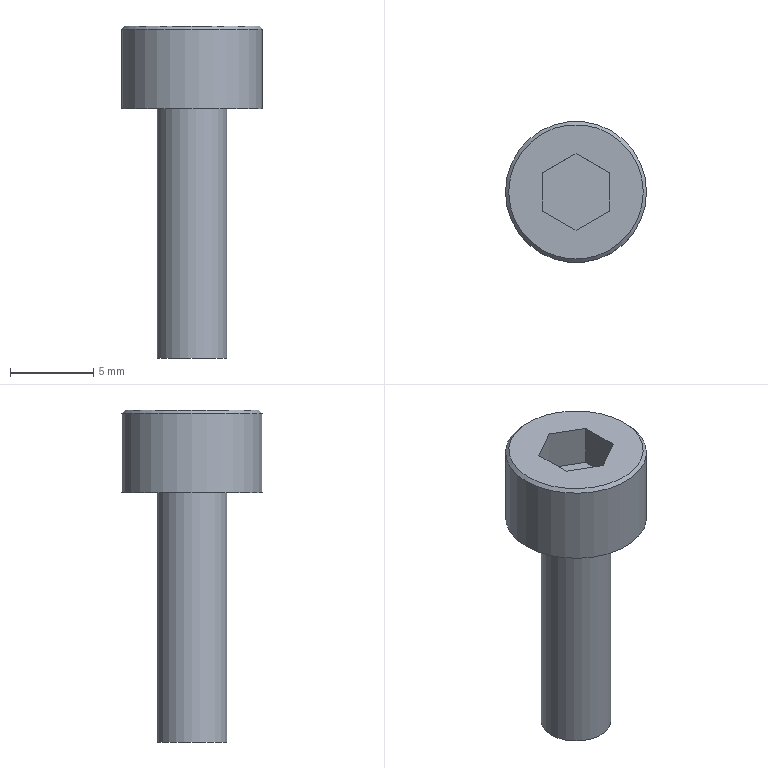Part | STEP file | M3-10_id34_x_t | 1 solid | 13 faces | box 8.5 x 8.5 x 20 mm | volume 456.375 mm3 | plane 10 | cylinder 2 | cone 1 | commonest cylinder face diameters 4.2 x1 8.5 x1
STEP:
#1=CARTESIAN_POINT('',(-234.55,-47.,-11.));
#2=VERTEX_POINT('',#1);
#3=CARTESIAN_POINT('',(-232.45,-47.,-11.));
#4=DIRECTION('',(0.,0.,-1.));
#5=DIRECTION('',(-1.,0.,0.));
#6=AXIS2_PLACEMENT_3D('',#3,#4,#5);
#7=CIRCLE('',#6,2.1);
#8=EDGE_CURVE('',#2,#2,#7,.T.);
#9=ORIENTED_EDGE('',*,*,#8,.F.);
#10=EDGE_LOOP('',(#9));
#11=FACE_BOUND('',#10,.T.);
#12=CARTESIAN_POINT('',(-228.2,-47.,-11.));
#13=VERTEX_POINT('',#12);
#14=CARTESIAN_POINT('',(-232.45,-47.,-11.));
#15=DIRECTION('',(0.,0.,1.));
#16=DIRECTION('',(1.,0.,0.));
#17=AXIS2_PLACEMENT_3D('',#14,#15,#16);
#18=CIRCLE('',#17,4.25);
#19=EDGE_CURVE('',#13,#13,#18,.T.);
#20=ORIENTED_EDGE('',*,*,#19,.F.);
#21=EDGE_LOOP('',(#20));
#22=FACE_BOUND('',#21,.T.);
#23=CARTESIAN_POINT('',(-232.45,-47.,-11.));
#24=DIRECTION('',(0.,0.,-1.));
#25=DIRECTION('',(-1.,0.,0.));
#26=AXIS2_PLACEMENT_3D('',#23,#24,#25);
#27=PLANE('',#26);
#28=ADVANCED_FACE('',(#11,#22),#27,.T.);
#29=CARTESIAN_POINT('',(-230.35,-47.,-26.));
#30=VERTEX_POINT('',#29);
#31=CARTESIAN_POINT('',(-232.45,-47.,-26.));
#32=DIRECTION('',(0.,0.,1.));
#33=DIRECTION('',(1.,0.,0.));
#34=AXIS2_PLACEMENT_3D('',#31,#32,#33);
#35=CIRCLE('',#34,2.1);
#36=EDGE_CURVE('',#30,#30,#35,.T.);
#37=ORIENTED_EDGE('',*,*,#36,.F.);
#38=EDGE_LOOP('',(#37));
#39=FACE_OUTER_BOUND('',#38,.T.);
#40=CARTESIAN_POINT('',(-232.45,-47.,-26.));
#41=DIRECTION('',(0.,0.,-1.));
#42=DIRECTION('',(-1.,0.,0.));
#43=AXIS2_PLACEMENT_3D('',#40,#41,#42);
#44=PLANE('',#43);
#45=ADVANCED_FACE('',(#39),#44,.T.);
#46=ORIENTED_EDGE('',*,*,#36,.T.);
#47=EDGE_LOOP('',(#46));
#48=FACE_BOUND('',#47,.T.);
#49=ORIENTED_EDGE('',*,*,#8,.T.);
#50=EDGE_LOOP('',(#49));
#51=FACE_BOUND('',#50,.T.);
#52=CARTESIAN_POINT('',(-232.45,-47.,-16.));
#53=DIRECTION('',(0.,0.,-1.));
#54=DIRECTION('',(1.,0.,0.));
#55=AXIS2_PLACEMENT_3D('',#52,#53,#54);
#56=CYLINDRICAL_SURFACE('',#55,2.1);
#57=ADVANCED_FACE('',(#48,#51),#56,.T.);
#58=CARTESIAN_POINT('',(-234.45,-45.845,-6.));
#59=VERTEX_POINT('',#58);
#60=CARTESIAN_POINT('',(-234.45,-48.155,-6.));
#61=VERTEX_POINT('',#60);
#62=CARTESIAN_POINT('',(-234.45,-45.845,-6.));
#63=DIRECTION('',(0.,-1.,0.));
#64=VECTOR('',#63,1.);
#65=LINE('',#62,#64);
#66=EDGE_CURVE('',#59,#61,#65,.T.);
#67=ORIENTED_EDGE('',*,*,#66,.F.);
#68=CARTESIAN_POINT('',(-232.45,-44.691,-6.));
#69=VERTEX_POINT('',#68);
#70=CARTESIAN_POINT('',(-232.45,-44.691,-6.));
#71=DIRECTION('',(-0.866,-0.5,0.));
#72=VECTOR('',#71,1.);
#73=LINE('',#70,#72);
#74=EDGE_CURVE('',#69,#59,#73,.T.);
#75=ORIENTED_EDGE('',*,*,#74,.F.);
#76=CARTESIAN_POINT('',(-230.45,-45.845,-6.));
#77=VERTEX_POINT('',#76);
#78=CARTESIAN_POINT('',(-230.45,-45.845,-6.));
#79=DIRECTION('',(-0.866,0.5,0.));
#80=VECTOR('',#79,1.);
#81=LINE('',#78,#80);
#82=EDGE_CURVE('',#77,#69,#81,.T.);
#83=ORIENTED_EDGE('',*,*,#82,.F.);
#84=CARTESIAN_POINT('',(-230.45,-48.155,-6.));
#85=VERTEX_POINT('',#84);
#86=CARTESIAN_POINT('',(-230.45,-48.155,-6.));
#87=DIRECTION('',(0.,1.,0.));
#88=VECTOR('',#87,1.);
#89=LINE('',#86,#88);
#90=EDGE_CURVE('',#85,#77,#89,.T.);
#91=ORIENTED_EDGE('',*,*,#90,.F.);
#92=CARTESIAN_POINT('',(-232.45,-49.309,-6.));
#93=VERTEX_POINT('',#92);
#94=CARTESIAN_POINT('',(-232.45,-49.309,-6.));
#95=DIRECTION('',(0.866,0.5,0.));
#96=VECTOR('',#95,1.);
#97=LINE('',#94,#96);
#98=EDGE_CURVE('',#93,#85,#97,.T.);
#99=ORIENTED_EDGE('',*,*,#98,.F.);
#100=CARTESIAN_POINT('',(-234.45,-48.155,-6.));
#101=DIRECTION('',(0.866,-0.5,0.));
#102=VECTOR('',#101,1.);
#103=LINE('',#100,#102);
#104=EDGE_CURVE('',#61,#93,#103,.T.);
#105=ORIENTED_EDGE('',*,*,#104,.F.);
#106=EDGE_LOOP('',(#67,#75,#83,#91,#99,#105));
#107=FACE_BOUND('',#106,.T.);
#108=CARTESIAN_POINT('',(-228.4,-47.,-6.));
#109=VERTEX_POINT('',#108);
#110=CARTESIAN_POINT('',(-232.45,-47.,-6.));
#111=DIRECTION('',(0.,0.,1.));
#112=DIRECTION('',(1.,0.,0.));
#113=AXIS2_PLACEMENT_3D('',#110,#111,#112);
#114=CIRCLE('',#113,4.05);
#115=EDGE_CURVE('',#109,#109,#114,.T.);
#116=ORIENTED_EDGE('',*,*,#115,.T.);
#117=EDGE_LOOP('',(#116));
#118=FACE_BOUND('',#117,.T.);
#119=CARTESIAN_POINT('',(-232.45,-47.,-6.));
#120=DIRECTION('',(0.,0.,1.));
#121=DIRECTION('',(1.,0.,0.));
#122=AXIS2_PLACEMENT_3D('',#119,#120,#121);
#123=PLANE('',#122);
#124=ADVANCED_FACE('',(#107,#118),#123,.T.);
#125=CARTESIAN_POINT('',(-228.2,-47.,-6.2));
#126=VERTEX_POINT('',#125);
#127=CARTESIAN_POINT('',(-232.45,-47.,-6.2));
#128=DIRECTION('',(0.,0.,-1.));
#129=DIRECTION('',(1.,0.,0.));
#130=AXIS2_PLACEMENT_3D('',#127,#128,#129);
#131=CIRCLE('',#130,4.25);
#132=EDGE_CURVE('',#126,#126,#131,.T.);
#133=ORIENTED_EDGE('',*,*,#132,.T.);
#134=EDGE_LOOP('',(#133));
#135=FACE_BOUND('',#134,.T.);
#136=ORIENTED_EDGE('',*,*,#19,.T.);
#137=EDGE_LOOP('',(#136));
#138=FACE_BOUND('',#137,.T.);
#139=CARTESIAN_POINT('',(-232.45,-47.,-11.));
#140=DIRECTION('',(0.,0.,1.));
#141=DIRECTION('',(1.,0.,0.));
#142=AXIS2_PLACEMENT_3D('',#139,#140,#141);
#143=CYLINDRICAL_SURFACE('',#142,4.25);
#144=ADVANCED_FACE('',(#135,#138),#143,.T.);
#145=ORIENTED_EDGE('',*,*,#115,.F.);
#146=EDGE_LOOP('',(#145));
#147=FACE_BOUND('',#146,.T.);
#148=ORIENTED_EDGE('',*,*,#132,.F.);
#149=EDGE_LOOP('',(#148));
#150=FACE_BOUND('',#149,.T.);
#151=CARTESIAN_POINT('',(-232.45,-47.,-6.2));
#152=DIRECTION('',(0.,0.,-1.));
#153=DIRECTION('',(-1.,0.,0.));
#154=AXIS2_PLACEMENT_3D('',#151,#152,#153);
#155=CONICAL_SURFACE('',#154,4.25,45.);
#156=ADVANCED_FACE('',(#147,#150),#155,.T.);
#157=ORIENTED_EDGE('',*,*,#66,.T.);
#158=CARTESIAN_POINT('',(-234.45,-48.155,-8.5));
#159=VERTEX_POINT('',#158);
#160=CARTESIAN_POINT('',(-234.45,-48.155,-8.5));
#161=DIRECTION('',(0.,0.,-1.));
#162=VECTOR('',#161,1.);
#163=LINE('',#160,#162);
#164=EDGE_CURVE('',#61,#159,#163,.T.);
#165=ORIENTED_EDGE('',*,*,#164,.T.);
#166=CARTESIAN_POINT('',(-234.45,-45.845,-8.5));
#167=VERTEX_POINT('',#166);
#168=CARTESIAN_POINT('',(-234.45,-45.845,-8.5));
#169=DIRECTION('',(0.,1.,0.));
#170=VECTOR('',#169,1.);
#171=LINE('',#168,#170);
#172=EDGE_CURVE('',#159,#167,#171,.T.);
#173=ORIENTED_EDGE('',*,*,#172,.T.);
#174=CARTESIAN_POINT('',(-234.45,-45.845,-8.5));
#175=DIRECTION('',(0.,0.,-1.));
#176=VECTOR('',#175,1.);
#177=LINE('',#174,#176);
#178=EDGE_CURVE('',#59,#167,#177,.T.);
#179=ORIENTED_EDGE('',*,*,#178,.F.);
#180=EDGE_LOOP('',(#157,#165,#173,#179));
#181=FACE_OUTER_BOUND('',#180,.T.);
#182=CARTESIAN_POINT('',(-234.45,-45.845,-8.5));
#183=DIRECTION('',(-1.,0.,0.));
#184=DIRECTION('',(0.,-1.,0.));
#185=AXIS2_PLACEMENT_3D('',#182,#183,#184);
#186=PLANE('',#185);
#187=ADVANCED_FACE('',(#181),#186,.F.);
#188=ORIENTED_EDGE('',*,*,#104,.T.);
#189=CARTESIAN_POINT('',(-232.45,-49.309,-8.5));
#190=VERTEX_POINT('',#189);
#191=CARTESIAN_POINT('',(-232.45,-49.309,-8.5));
#192=DIRECTION('',(0.,0.,-1.));
#193=VECTOR('',#192,1.);
#194=LINE('',#191,#193);
#195=EDGE_CURVE('',#93,#190,#194,.T.);
#196=ORIENTED_EDGE('',*,*,#195,.T.);
#197=CARTESIAN_POINT('',(-234.45,-48.155,-8.5));
#198=DIRECTION('',(-0.866,0.5,0.));
#199=VECTOR('',#198,1.);
#200=LINE('',#197,#199);
#201=EDGE_CURVE('',#190,#159,#200,.T.);
#202=ORIENTED_EDGE('',*,*,#201,.T.);
#203=ORIENTED_EDGE('',*,*,#164,.F.);
#204=EDGE_LOOP('',(#188,#196,#202,#203));
#205=FACE_OUTER_BOUND('',#204,.T.);
#206=CARTESIAN_POINT('',(-234.45,-48.155,-8.5));
#207=DIRECTION('',(-0.5,-0.866,0.));
#208=DIRECTION('',(0.866,-0.5,0.));
#209=AXIS2_PLACEMENT_3D('',#206,#207,#208);
#210=PLANE('',#209);
#211=ADVANCED_FACE('',(#205),#210,.F.);
#212=ORIENTED_EDGE('',*,*,#98,.T.);
#213=CARTESIAN_POINT('',(-230.45,-48.155,-8.5));
#214=VERTEX_POINT('',#213);
#215=CARTESIAN_POINT('',(-230.45,-48.155,-8.5));
#216=DIRECTION('',(0.,0.,-1.));
#217=VECTOR('',#216,1.);
#218=LINE('',#215,#217);
#219=EDGE_CURVE('',#85,#214,#218,.T.);
#220=ORIENTED_EDGE('',*,*,#219,.T.);
#221=CARTESIAN_POINT('',(-232.45,-49.309,-8.5));
#222=DIRECTION('',(-0.866,-0.5,0.));
#223=VECTOR('',#222,1.);
#224=LINE('',#221,#223);
#225=EDGE_CURVE('',#214,#190,#224,.T.);
#226=ORIENTED_EDGE('',*,*,#225,.T.);
#227=ORIENTED_EDGE('',*,*,#195,.F.);
#228=EDGE_LOOP('',(#212,#220,#226,#227));
#229=FACE_OUTER_BOUND('',#228,.T.);
#230=CARTESIAN_POINT('',(-232.45,-49.309,-8.5));
#231=DIRECTION('',(0.5,-0.866,0.));
#232=DIRECTION('',(0.866,0.5,0.));
#233=AXIS2_PLACEMENT_3D('',#230,#231,#232);
#234=PLANE('',#233);
#235=ADVANCED_FACE('',(#229),#234,.F.);
#236=ORIENTED_EDGE('',*,*,#90,.T.);
#237=CARTESIAN_POINT('',(-230.45,-45.845,-8.5));
#238=VERTEX_POINT('',#237);
#239=CARTESIAN_POINT('',(-230.45,-45.845,-8.5));
#240=DIRECTION('',(0.,0.,-1.));
#241=VECTOR('',#240,1.);
#242=LINE('',#239,#241);
#243=EDGE_CURVE('',#77,#238,#242,.T.);
#244=ORIENTED_EDGE('',*,*,#243,.T.);
#245=CARTESIAN_POINT('',(-230.45,-48.155,-8.5));
#246=DIRECTION('',(0.,-1.,0.));
#247=VECTOR('',#246,1.);
#248=LINE('',#245,#247);
#249=EDGE_CURVE('',#238,#214,#248,.T.);
#250=ORIENTED_EDGE('',*,*,#249,.T.);
#251=ORIENTED_EDGE('',*,*,#219,.F.);
#252=EDGE_LOOP('',(#236,#244,#250,#251));
#253=FACE_OUTER_BOUND('',#252,.T.);
#254=CARTESIAN_POINT('',(-230.45,-48.155,-8.5));
#255=DIRECTION('',(1.,0.,0.));
#256=DIRECTION('',(0.,1.,0.));
#257=AXIS2_PLACEMENT_3D('',#254,#255,#256);
#258=PLANE('',#257);
#259=ADVANCED_FACE('',(#253),#258,.F.);
#260=ORIENTED_EDGE('',*,*,#82,.T.);
#261=CARTESIAN_POINT('',(-232.45,-44.691,-8.5));
#262=VERTEX_POINT('',#261);
#263=CARTESIAN_POINT('',(-232.45,-44.691,-8.5));
#264=DIRECTION('',(0.,0.,-1.));
#265=VECTOR('',#264,1.);
#266=LINE('',#263,#265);
#267=EDGE_CURVE('',#69,#262,#266,.T.);
#268=ORIENTED_EDGE('',*,*,#267,.T.);
#269=CARTESIAN_POINT('',(-230.45,-45.845,-8.5));
#270=DIRECTION('',(0.866,-0.5,0.));
#271=VECTOR('',#270,1.);
#272=LINE('',#269,#271);
#273=EDGE_CURVE('',#262,#238,#272,.T.);
#274=ORIENTED_EDGE('',*,*,#273,.T.);
#275=ORIENTED_EDGE('',*,*,#243,.F.);
#276=EDGE_LOOP('',(#260,#268,#274,#275));
#277=FACE_OUTER_BOUND('',#276,.T.);
#278=CARTESIAN_POINT('',(-230.45,-45.845,-8.5));
#279=DIRECTION('',(0.5,0.866,0.));
#280=DIRECTION('',(-0.866,0.5,0.));
#281=AXIS2_PLACEMENT_3D('',#278,#279,#280);
#282=PLANE('',#281);
#283=ADVANCED_FACE('',(#277),#282,.F.);
#284=ORIENTED_EDGE('',*,*,#74,.T.);
#285=ORIENTED_EDGE('',*,*,#178,.T.);
#286=CARTESIAN_POINT('',(-232.45,-44.691,-8.5));
#287=DIRECTION('',(0.866,0.5,0.));
#288=VECTOR('',#287,1.);
#289=LINE('',#286,#288);
#290=EDGE_CURVE('',#167,#262,#289,.T.);
#291=ORIENTED_EDGE('',*,*,#290,.T.);
#292=ORIENTED_EDGE('',*,*,#267,.F.);
#293=EDGE_LOOP('',(#284,#285,#291,#292));
#294=FACE_OUTER_BOUND('',#293,.T.);
#295=CARTESIAN_POINT('',(-232.45,-44.691,-8.5));
#296=DIRECTION('',(-0.5,0.866,0.));
#297=DIRECTION('',(-0.866,-0.5,0.));
#298=AXIS2_PLACEMENT_3D('',#295,#296,#297);
#299=PLANE('',#298);
#300=ADVANCED_FACE('',(#294),#299,.F.);
#301=ORIENTED_EDGE('',*,*,#172,.F.);
#302=ORIENTED_EDGE('',*,*,#201,.F.);
#303=ORIENTED_EDGE('',*,*,#225,.F.);
#304=ORIENTED_EDGE('',*,*,#249,.F.);
#305=ORIENTED_EDGE('',*,*,#273,.F.);
#306=ORIENTED_EDGE('',*,*,#290,.F.);
#307=EDGE_LOOP('',(#301,#302,#303,#304,#305,#306));
#308=FACE_OUTER_BOUND('',#307,.T.);
#309=CARTESIAN_POINT('',(-232.45,-47.,-8.5));
#310=DIRECTION('',(0.,0.,1.));
#311=DIRECTION('',(1.,0.,0.));
#312=AXIS2_PLACEMENT_3D('',#309,#310,#311);
#313=PLANE('',#312);
#314=ADVANCED_FACE('',(#308),#313,.T.);
#315=CLOSED_SHELL('',(#28,#45,#57,#124,#144,#156,#187,#211,#235,#259,#283,#300,#314));
#316=MANIFOLD_SOLID_BREP('',#315);
#317=(LENGTH_UNIT()NAMED_UNIT(*)SI_UNIT(.MILLI.,.METRE.));
#318=UNCERTAINTY_MEASURE_WITH_UNIT(LENGTH_MEASURE(0.00002),#317,'','');
#319=(NAMED_UNIT(*)PLANE_ANGLE_UNIT()SI_UNIT($,.RADIAN.));
#320=PLANE_ANGLE_MEASURE_WITH_UNIT(PLANE_ANGLE_MEASURE(0.01745),#319);
#321=DIMENSIONAL_EXPONENTS(0.,0.,0.,0.,0.,0.,0.);
#322=(CONVERSION_BASED_UNIT('DEGREE',#320)NAMED_UNIT(#321)PLANE_ANGLE_UNIT());
#323=(NAMED_UNIT(*)SI_UNIT($,.STERADIAN.)SOLID_ANGLE_UNIT());
#324=(GEOMETRIC_REPRESENTATION_CONTEXT(3)GLOBAL_UNCERTAINTY_ASSIGNED_CONTEXT((#318))GLOBAL_UNIT_ASSIGNED_CONTEXT((#317,#322,#323))REPRESENTATION_CONTEXT('',''));
#325=ADVANCED_BREP_SHAPE_REPRESENTATION('',(#316),#324);